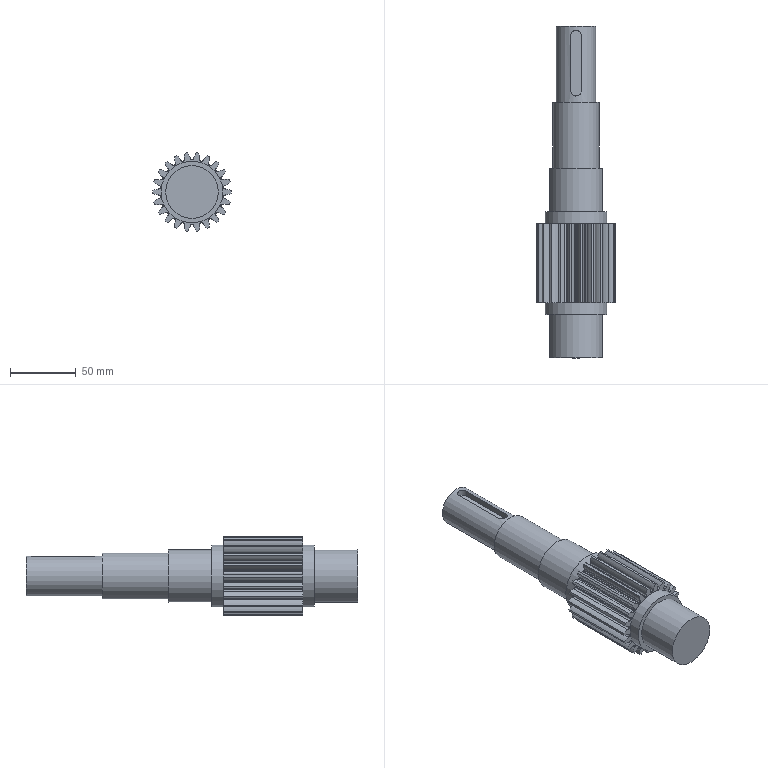Part | NX | features BREP 22, META 22, DATUM_CSYS 8, EXTRUDE 7, SKETCH 7, EXTRACT_DATUM_AXIS 2, EXTRACT_DATUM_PLANE 2, BLEND 1, CYLINDER 1, FSET 1, Instance Feature 1, Mirror Feature 1 | 6 solids | 156 faces | box 60 x 252 x 59.615 mm | volume 341814 mm3 | spline 110 | cylinder 30 | plane 16 | commonest cylinder face diameters 48.75 x22 8 x2 40 x2 47 x2 30 x1 35 x1